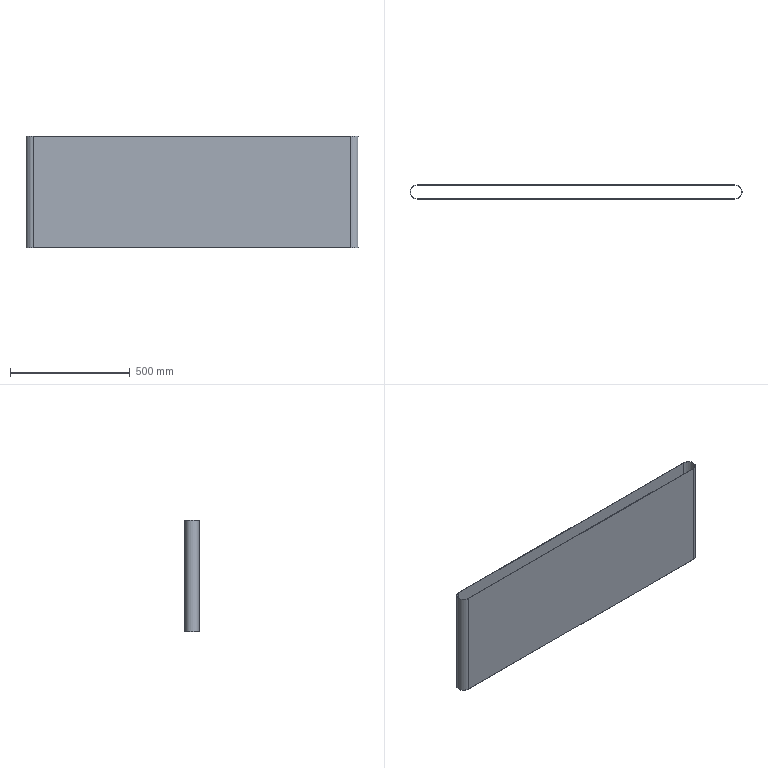Part | STEP file | RUBE 601 | 1 solid | 10 faces | box 1389 x 59.2 x 465 mm | volume 2113671 mm3 | plane 6 | cylinder 4 | commonest cylinder face diameters 56 x2 59.2 x2
STEP:
#1=CARTESIAN_POINT('',(0.,0.,0.));
#2=DIRECTION('',(0.,0.,1.));
#3=DIRECTION('',(1.,0.,0.));
#4=AXIS2_PLACEMENT_3D('',#1,#2,#3);
#5=CARTESIAN_POINT('',(-1248.5,29.6,232.5));
#6=VERTEX_POINT('',#5);
#7=CARTESIAN_POINT('',(-1248.5,-29.6,232.5));
#8=VERTEX_POINT('',#7);
#9=CARTESIAN_POINT('',(-1248.5,0.,232.5));
#10=DIRECTION('',(0.,0.,1.));
#11=DIRECTION('',(1.,0.,0.));
#12=AXIS2_PLACEMENT_3D('',#9,#10,#11);
#13=CIRCLE('',#12,29.6);
#14=CARTESIAN_POINT('',(-1248.5,0.,232.5));
#15=DIRECTION('',(0.,0.,1.));
#16=DIRECTION('',(1.,0.,0.));
#17=AXIS2_PLACEMENT_3D('',#14,#15,#16);
#18=PLANE('',#17);
#19=CARTESIAN_POINT('',(0.,0.));
#20=DIRECTION('',(1.,0.));
#21=AXIS2_PLACEMENT_2D('',#19,#20);
#22=CIRCLE('',#21,29.6);
#23=(GEOMETRIC_REPRESENTATION_CONTEXT(2)PARAMETRIC_REPRESENTATION_CONTEXT()REPRESENTATION_CONTEXT('',''));
#24=DEFINITIONAL_REPRESENTATION('',(#22),#23);
#25=PCURVE('',#18,#24);
#26=CARTESIAN_POINT('',(-1248.5,0.,232.5));
#27=DIRECTION('',(0.,0.,-1.));
#28=DIRECTION('',(-1.,0.,0.));
#29=AXIS2_PLACEMENT_3D('',#26,#27,#28);
#30=CYLINDRICAL_SURFACE('',#29,29.6);
#31=CARTESIAN_POINT('',(3.142,0.));
#32=DIRECTION('',(-1.,0.));
#33=VECTOR('',#32,1.);
#34=LINE('',#31,#33);
#35=(GEOMETRIC_REPRESENTATION_CONTEXT(2)PARAMETRIC_REPRESENTATION_CONTEXT()REPRESENTATION_CONTEXT('',''));
#36=DEFINITIONAL_REPRESENTATION('',(#34),#35);
#37=PCURVE('',#30,#36);
#38=SURFACE_CURVE('',#13,(#25,#37),.PCURVE_S1.);
#39=EDGE_CURVE('',#6,#8,#38,.T.);
#40=ORIENTED_EDGE('',*,*,#39,.T.);
#41=CARTESIAN_POINT('',(81.5,-29.6,232.5));
#42=VERTEX_POINT('',#41);
#43=CARTESIAN_POINT('',(-1248.5,-29.6,232.5));
#44=DIRECTION('',(1.,0.,0.));
#45=VECTOR('',#44,1.);
#46=LINE('',#43,#45);
#47=CARTESIAN_POINT('',(0.,-29.6));
#48=DIRECTION('',(1.,0.));
#49=VECTOR('',#48,1.);
#50=LINE('',#47,#49);
#51=(GEOMETRIC_REPRESENTATION_CONTEXT(2)PARAMETRIC_REPRESENTATION_CONTEXT()REPRESENTATION_CONTEXT('',''));
#52=DEFINITIONAL_REPRESENTATION('',(#50),#51);
#53=PCURVE('',#18,#52);
#54=CARTESIAN_POINT('',(-1248.5,-29.6,232.5));
#55=DIRECTION('',(0.,1.,0.));
#56=DIRECTION('',(-1.,0.,0.));
#57=AXIS2_PLACEMENT_3D('',#54,#55,#56);
#58=PLANE('',#57);
#59=CARTESIAN_POINT('',(0.,0.));
#60=DIRECTION('',(-1.,0.));
#61=VECTOR('',#60,1.);
#62=LINE('',#59,#61);
#63=(GEOMETRIC_REPRESENTATION_CONTEXT(2)PARAMETRIC_REPRESENTATION_CONTEXT()REPRESENTATION_CONTEXT('',''));
#64=DEFINITIONAL_REPRESENTATION('',(#62),#63);
#65=PCURVE('',#58,#64);
#66=SURFACE_CURVE('',#46,(#53,#65),.PCURVE_S1.);
#67=EDGE_CURVE('',#8,#42,#66,.T.);
#68=ORIENTED_EDGE('',*,*,#67,.T.);
#69=CARTESIAN_POINT('',(81.5,29.6,232.5));
#70=VERTEX_POINT('',#69);
#71=CARTESIAN_POINT('',(81.5,0.,232.5));
#72=DIRECTION('',(0.,0.,1.));
#73=DIRECTION('',(1.,0.,0.));
#74=AXIS2_PLACEMENT_3D('',#71,#72,#73);
#75=CIRCLE('',#74,29.6);
#76=CARTESIAN_POINT('',(1330.,0.));
#77=DIRECTION('',(1.,0.));
#78=AXIS2_PLACEMENT_2D('',#76,#77);
#79=CIRCLE('',#78,29.6);
#80=(GEOMETRIC_REPRESENTATION_CONTEXT(2)PARAMETRIC_REPRESENTATION_CONTEXT()REPRESENTATION_CONTEXT('',''));
#81=DEFINITIONAL_REPRESENTATION('',(#79),#80);
#82=PCURVE('',#18,#81);
#83=CARTESIAN_POINT('',(81.5,0.,232.5));
#84=DIRECTION('',(0.,0.,-1.));
#85=DIRECTION('',(-1.,0.,0.));
#86=AXIS2_PLACEMENT_3D('',#83,#84,#85);
#87=CYLINDRICAL_SURFACE('',#86,29.6);
#88=CARTESIAN_POINT('',(9.425,0.));
#89=DIRECTION('',(-1.,0.));
#90=VECTOR('',#89,1.);
#91=LINE('',#88,#90);
#92=(GEOMETRIC_REPRESENTATION_CONTEXT(2)PARAMETRIC_REPRESENTATION_CONTEXT()REPRESENTATION_CONTEXT('',''));
#93=DEFINITIONAL_REPRESENTATION('',(#91),#92);
#94=PCURVE('',#87,#93);
#95=SURFACE_CURVE('',#75,(#82,#94),.PCURVE_S1.);
#96=EDGE_CURVE('',#42,#70,#95,.T.);
#97=ORIENTED_EDGE('',*,*,#96,.T.);
#98=CARTESIAN_POINT('',(-1248.5,29.6,232.5));
#99=DIRECTION('',(-1.,0.,0.));
#100=VECTOR('',#99,1.);
#101=LINE('',#98,#100);
#102=CARTESIAN_POINT('',(0.,29.6));
#103=DIRECTION('',(-1.,0.));
#104=VECTOR('',#103,1.);
#105=LINE('',#102,#104);
#106=(GEOMETRIC_REPRESENTATION_CONTEXT(2)PARAMETRIC_REPRESENTATION_CONTEXT()REPRESENTATION_CONTEXT('',''));
#107=DEFINITIONAL_REPRESENTATION('',(#105),#106);
#108=PCURVE('',#18,#107);
#109=CARTESIAN_POINT('',(-1248.5,29.6,232.5));
#110=DIRECTION('',(0.,-1.,0.));
#111=DIRECTION('',(1.,0.,0.));
#112=AXIS2_PLACEMENT_3D('',#109,#110,#111);
#113=PLANE('',#112);
#114=CARTESIAN_POINT('',(0.,0.));
#115=DIRECTION('',(-1.,0.));
#116=VECTOR('',#115,1.);
#117=LINE('',#114,#116);
#118=(GEOMETRIC_REPRESENTATION_CONTEXT(2)PARAMETRIC_REPRESENTATION_CONTEXT()REPRESENTATION_CONTEXT('',''));
#119=DEFINITIONAL_REPRESENTATION('',(#117),#118);
#120=PCURVE('',#113,#119);
#121=SURFACE_CURVE('',#101,(#108,#120),.PCURVE_S1.);
#122=EDGE_CURVE('',#70,#6,#121,.T.);
#123=ORIENTED_EDGE('',*,*,#122,.T.);
#124=EDGE_LOOP('',(#40,#68,#97,#123));
#125=FACE_BOUND('',#124,.T.);
#126=CARTESIAN_POINT('',(-1248.5,-28.,232.5));
#127=VERTEX_POINT('',#126);
#128=CARTESIAN_POINT('',(81.5,-28.,232.5));
#129=VERTEX_POINT('',#128);
#130=CARTESIAN_POINT('',(-1248.5,-28.,232.5));
#131=DIRECTION('',(1.,0.,0.));
#132=VECTOR('',#131,1.);
#133=LINE('',#130,#132);
#134=CARTESIAN_POINT('',(0.,-28.));
#135=DIRECTION('',(1.,0.));
#136=VECTOR('',#135,1.);
#137=LINE('',#134,#136);
#138=(GEOMETRIC_REPRESENTATION_CONTEXT(2)PARAMETRIC_REPRESENTATION_CONTEXT()REPRESENTATION_CONTEXT('',''));
#139=DEFINITIONAL_REPRESENTATION('',(#137),#138);
#140=PCURVE('',#18,#139);
#141=CARTESIAN_POINT('',(-1248.5,-28.,232.5));
#142=DIRECTION('',(0.,1.,0.));
#143=DIRECTION('',(-1.,0.,0.));
#144=AXIS2_PLACEMENT_3D('',#141,#142,#143);
#145=PLANE('',#144);
#146=CARTESIAN_POINT('',(0.,0.));
#147=DIRECTION('',(-1.,0.));
#148=VECTOR('',#147,1.);
#149=LINE('',#146,#148);
#150=(GEOMETRIC_REPRESENTATION_CONTEXT(2)PARAMETRIC_REPRESENTATION_CONTEXT()REPRESENTATION_CONTEXT('',''));
#151=DEFINITIONAL_REPRESENTATION('',(#149),#150);
#152=PCURVE('',#145,#151);
#153=SURFACE_CURVE('',#133,(#140,#152),.PCURVE_S1.);
#154=EDGE_CURVE('',#127,#129,#153,.T.);
#155=ORIENTED_EDGE('',*,*,#154,.F.);
#156=CARTESIAN_POINT('',(-1248.5,28.,232.5));
#157=VERTEX_POINT('',#156);
#158=CARTESIAN_POINT('',(-1248.5,0.,232.5));
#159=DIRECTION('',(0.,0.,1.));
#160=DIRECTION('',(1.,0.,0.));
#161=AXIS2_PLACEMENT_3D('',#158,#159,#160);
#162=CIRCLE('',#161,28.);
#163=CARTESIAN_POINT('',(0.,0.));
#164=DIRECTION('',(1.,0.));
#165=AXIS2_PLACEMENT_2D('',#163,#164);
#166=CIRCLE('',#165,28.);
#167=(GEOMETRIC_REPRESENTATION_CONTEXT(2)PARAMETRIC_REPRESENTATION_CONTEXT()REPRESENTATION_CONTEXT('',''));
#168=DEFINITIONAL_REPRESENTATION('',(#166),#167);
#169=PCURVE('',#18,#168);
#170=CARTESIAN_POINT('',(-1248.5,0.,232.5));
#171=DIRECTION('',(0.,0.,-1.));
#172=DIRECTION('',(-1.,0.,0.));
#173=AXIS2_PLACEMENT_3D('',#170,#171,#172);
#174=CYLINDRICAL_SURFACE('',#173,28.);
#175=CARTESIAN_POINT('',(9.425,0.));
#176=DIRECTION('',(-1.,0.));
#177=VECTOR('',#176,1.);
#178=LINE('',#175,#177);
#179=(GEOMETRIC_REPRESENTATION_CONTEXT(2)PARAMETRIC_REPRESENTATION_CONTEXT()REPRESENTATION_CONTEXT('',''));
#180=DEFINITIONAL_REPRESENTATION('',(#178),#179);
#181=PCURVE('',#174,#180);
#182=SURFACE_CURVE('',#162,(#169,#181),.PCURVE_S1.);
#183=EDGE_CURVE('',#157,#127,#182,.T.);
#184=ORIENTED_EDGE('',*,*,#183,.F.);
#185=CARTESIAN_POINT('',(81.5,28.,232.5));
#186=VERTEX_POINT('',#185);
#187=CARTESIAN_POINT('',(-1248.5,28.,232.5));
#188=DIRECTION('',(-1.,0.,0.));
#189=VECTOR('',#188,1.);
#190=LINE('',#187,#189);
#191=CARTESIAN_POINT('',(0.,28.));
#192=DIRECTION('',(-1.,0.));
#193=VECTOR('',#192,1.);
#194=LINE('',#191,#193);
#195=(GEOMETRIC_REPRESENTATION_CONTEXT(2)PARAMETRIC_REPRESENTATION_CONTEXT()REPRESENTATION_CONTEXT('',''));
#196=DEFINITIONAL_REPRESENTATION('',(#194),#195);
#197=PCURVE('',#18,#196);
#198=CARTESIAN_POINT('',(-1248.5,28.,232.5));
#199=DIRECTION('',(0.,-1.,0.));
#200=DIRECTION('',(1.,0.,0.));
#201=AXIS2_PLACEMENT_3D('',#198,#199,#200);
#202=PLANE('',#201);
#203=CARTESIAN_POINT('',(0.,0.));
#204=DIRECTION('',(-1.,0.));
#205=VECTOR('',#204,1.);
#206=LINE('',#203,#205);
#207=(GEOMETRIC_REPRESENTATION_CONTEXT(2)PARAMETRIC_REPRESENTATION_CONTEXT()REPRESENTATION_CONTEXT('',''));
#208=DEFINITIONAL_REPRESENTATION('',(#206),#207);
#209=PCURVE('',#202,#208);
#210=SURFACE_CURVE('',#190,(#197,#209),.PCURVE_S1.);
#211=EDGE_CURVE('',#186,#157,#210,.T.);
#212=ORIENTED_EDGE('',*,*,#211,.F.);
#213=CARTESIAN_POINT('',(81.5,0.,232.5));
#214=DIRECTION('',(0.,0.,1.));
#215=DIRECTION('',(1.,0.,0.));
#216=AXIS2_PLACEMENT_3D('',#213,#214,#215);
#217=CIRCLE('',#216,28.);
#218=CARTESIAN_POINT('',(1330.,0.));
#219=DIRECTION('',(1.,0.));
#220=AXIS2_PLACEMENT_2D('',#218,#219);
#221=CIRCLE('',#220,28.);
#222=(GEOMETRIC_REPRESENTATION_CONTEXT(2)PARAMETRIC_REPRESENTATION_CONTEXT()REPRESENTATION_CONTEXT('',''));
#223=DEFINITIONAL_REPRESENTATION('',(#221),#222);
#224=PCURVE('',#18,#223);
#225=CARTESIAN_POINT('',(81.5,0.,232.5));
#226=DIRECTION('',(0.,0.,-1.));
#227=DIRECTION('',(-1.,0.,0.));
#228=AXIS2_PLACEMENT_3D('',#225,#226,#227);
#229=CYLINDRICAL_SURFACE('',#228,28.);
#230=CARTESIAN_POINT('',(9.425,0.));
#231=DIRECTION('',(-1.,0.));
#232=VECTOR('',#231,1.);
#233=LINE('',#230,#232);
#234=(GEOMETRIC_REPRESENTATION_CONTEXT(2)PARAMETRIC_REPRESENTATION_CONTEXT()REPRESENTATION_CONTEXT('',''));
#235=DEFINITIONAL_REPRESENTATION('',(#233),#234);
#236=PCURVE('',#229,#235);
#237=SURFACE_CURVE('',#217,(#224,#236),.PCURVE_S1.);
#238=EDGE_CURVE('',#129,#186,#237,.T.);
#239=ORIENTED_EDGE('',*,*,#238,.F.);
#240=EDGE_LOOP('',(#155,#184,#212,#239));
#241=FACE_BOUND('',#240,.T.);
#242=ADVANCED_FACE('',(#125,#241),#18,.T.);
#243=CARTESIAN_POINT('',(-1248.5,29.6,-232.5));
#244=VERTEX_POINT('',#243);
#245=CARTESIAN_POINT('',(-1248.5,-29.6,-232.5));
#246=VERTEX_POINT('',#245);
#247=CARTESIAN_POINT('',(-1248.5,0.,-232.5));
#248=DIRECTION('',(0.,0.,1.));
#249=DIRECTION('',(1.,0.,0.));
#250=AXIS2_PLACEMENT_3D('',#247,#248,#249);
#251=CIRCLE('',#250,29.6);
#252=CARTESIAN_POINT('',(-1248.5,0.,-232.5));
#253=DIRECTION('',(0.,0.,1.));
#254=DIRECTION('',(1.,0.,0.));
#255=AXIS2_PLACEMENT_3D('',#252,#253,#254);
#256=PLANE('',#255);
#257=CARTESIAN_POINT('',(0.,0.));
#258=DIRECTION('',(1.,0.));
#259=AXIS2_PLACEMENT_2D('',#257,#258);
#260=CIRCLE('',#259,29.6);
#261=(GEOMETRIC_REPRESENTATION_CONTEXT(2)PARAMETRIC_REPRESENTATION_CONTEXT()REPRESENTATION_CONTEXT('',''));
#262=DEFINITIONAL_REPRESENTATION('',(#260),#261);
#263=PCURVE('',#256,#262);
#264=CARTESIAN_POINT('',(3.142,465.));
#265=DIRECTION('',(-1.,0.));
#266=VECTOR('',#265,1.);
#267=LINE('',#264,#266);
#268=(GEOMETRIC_REPRESENTATION_CONTEXT(2)PARAMETRIC_REPRESENTATION_CONTEXT()REPRESENTATION_CONTEXT('',''));
#269=DEFINITIONAL_REPRESENTATION('',(#267),#268);
#270=PCURVE('',#30,#269);
#271=SURFACE_CURVE('',#251,(#263,#270),.PCURVE_S1.);
#272=EDGE_CURVE('',#244,#246,#271,.T.);
#273=ORIENTED_EDGE('',*,*,#272,.F.);
#274=CARTESIAN_POINT('',(81.5,29.6,-232.5));
#275=VERTEX_POINT('',#274);
#276=CARTESIAN_POINT('',(-1248.5,29.6,-232.5));
#277=DIRECTION('',(-1.,0.,0.));
#278=VECTOR('',#277,1.);
#279=LINE('',#276,#278);
#280=CARTESIAN_POINT('',(0.,29.6));
#281=DIRECTION('',(-1.,0.));
#282=VECTOR('',#281,1.);
#283=LINE('',#280,#282);
#284=(GEOMETRIC_REPRESENTATION_CONTEXT(2)PARAMETRIC_REPRESENTATION_CONTEXT()REPRESENTATION_CONTEXT('',''));
#285=DEFINITIONAL_REPRESENTATION('',(#283),#284);
#286=PCURVE('',#256,#285);
#287=CARTESIAN_POINT('',(0.,-465.));
#288=DIRECTION('',(-1.,0.));
#289=VECTOR('',#288,1.);
#290=LINE('',#287,#289);
#291=(GEOMETRIC_REPRESENTATION_CONTEXT(2)PARAMETRIC_REPRESENTATION_CONTEXT()REPRESENTATION_CONTEXT('',''));
#292=DEFINITIONAL_REPRESENTATION('',(#290),#291);
#293=PCURVE('',#113,#292);
#294=SURFACE_CURVE('',#279,(#286,#293),.PCURVE_S1.);
#295=EDGE_CURVE('',#275,#244,#294,.T.);
#296=ORIENTED_EDGE('',*,*,#295,.F.);
#297=CARTESIAN_POINT('',(81.5,-29.6,-232.5));
#298=VERTEX_POINT('',#297);
#299=CARTESIAN_POINT('',(81.5,0.,-232.5));
#300=DIRECTION('',(0.,0.,1.));
#301=DIRECTION('',(1.,0.,0.));
#302=AXIS2_PLACEMENT_3D('',#299,#300,#301);
#303=CIRCLE('',#302,29.6);
#304=CARTESIAN_POINT('',(1330.,0.));
#305=DIRECTION('',(1.,0.));
#306=AXIS2_PLACEMENT_2D('',#304,#305);
#307=CIRCLE('',#306,29.6);
#308=(GEOMETRIC_REPRESENTATION_CONTEXT(2)PARAMETRIC_REPRESENTATION_CONTEXT()REPRESENTATION_CONTEXT('',''));
#309=DEFINITIONAL_REPRESENTATION('',(#307),#308);
#310=PCURVE('',#256,#309);
#311=CARTESIAN_POINT('',(9.425,465.));
#312=DIRECTION('',(-1.,0.));
#313=VECTOR('',#312,1.);
#314=LINE('',#311,#313);
#315=(GEOMETRIC_REPRESENTATION_CONTEXT(2)PARAMETRIC_REPRESENTATION_CONTEXT()REPRESENTATION_CONTEXT('',''));
#316=DEFINITIONAL_REPRESENTATION('',(#314),#315);
#317=PCURVE('',#87,#316);
#318=SURFACE_CURVE('',#303,(#310,#317),.PCURVE_S1.);
#319=EDGE_CURVE('',#298,#275,#318,.T.);
#320=ORIENTED_EDGE('',*,*,#319,.F.);
#321=CARTESIAN_POINT('',(-1248.5,-29.6,-232.5));
#322=DIRECTION('',(1.,0.,0.));
#323=VECTOR('',#322,1.);
#324=LINE('',#321,#323);
#325=CARTESIAN_POINT('',(0.,-29.6));
#326=DIRECTION('',(1.,0.));
#327=VECTOR('',#326,1.);
#328=LINE('',#325,#327);
#329=(GEOMETRIC_REPRESENTATION_CONTEXT(2)PARAMETRIC_REPRESENTATION_CONTEXT()REPRESENTATION_CONTEXT('',''));
#330=DEFINITIONAL_REPRESENTATION('',(#328),#329);
#331=PCURVE('',#256,#330);
#332=CARTESIAN_POINT('',(0.,-465.));
#333=DIRECTION('',(-1.,0.));
#334=VECTOR('',#333,1.);
#335=LINE('',#332,#334);
#336=(GEOMETRIC_REPRESENTATION_CONTEXT(2)PARAMETRIC_REPRESENTATION_CONTEXT()REPRESENTATION_CONTEXT('',''));
#337=DEFINITIONAL_REPRESENTATION('',(#335),#336);
#338=PCURVE('',#58,#337);
#339=SURFACE_CURVE('',#324,(#331,#338),.PCURVE_S1.);
#340=EDGE_CURVE('',#246,#298,#339,.T.);
#341=ORIENTED_EDGE('',*,*,#340,.F.);
#342=EDGE_LOOP('',(#273,#296,#320,#341));
#343=FACE_BOUND('',#342,.T.);
#344=CARTESIAN_POINT('',(-1248.5,28.,-232.5));
#345=VERTEX_POINT('',#344);
#346=CARTESIAN_POINT('',(-1248.5,-28.,-232.5));
#347=VERTEX_POINT('',#346);
#348=CARTESIAN_POINT('',(-1248.5,0.,-232.5));
#349=DIRECTION('',(0.,0.,1.));
#350=DIRECTION('',(1.,0.,0.));
#351=AXIS2_PLACEMENT_3D('',#348,#349,#350);
#352=CIRCLE('',#351,28.);
#353=CARTESIAN_POINT('',(0.,0.));
#354=DIRECTION('',(1.,0.));
#355=AXIS2_PLACEMENT_2D('',#353,#354);
#356=CIRCLE('',#355,28.);
#357=(GEOMETRIC_REPRESENTATION_CONTEXT(2)PARAMETRIC_REPRESENTATION_CONTEXT()REPRESENTATION_CONTEXT('',''));
#358=DEFINITIONAL_REPRESENTATION('',(#356),#357);
#359=PCURVE('',#256,#358);
#360=CARTESIAN_POINT('',(9.425,465.));
#361=DIRECTION('',(-1.,0.));
#362=VECTOR('',#361,1.);
#363=LINE('',#360,#362);
#364=(GEOMETRIC_REPRESENTATION_CONTEXT(2)PARAMETRIC_REPRESENTATION_CONTEXT()REPRESENTATION_CONTEXT('',''));
#365=DEFINITIONAL_REPRESENTATION('',(#363),#364);
#366=PCURVE('',#174,#365);
#367=SURFACE_CURVE('',#352,(#359,#366),.PCURVE_S1.);
#368=EDGE_CURVE('',#345,#347,#367,.T.);
#369=ORIENTED_EDGE('',*,*,#368,.T.);
#370=CARTESIAN_POINT('',(81.5,-28.,-232.5));
#371=VERTEX_POINT('',#370);
#372=CARTESIAN_POINT('',(-1248.5,-28.,-232.5));
#373=DIRECTION('',(1.,0.,0.));
#374=VECTOR('',#373,1.);
#375=LINE('',#372,#374);
#376=CARTESIAN_POINT('',(0.,-28.));
#377=DIRECTION('',(1.,0.));
#378=VECTOR('',#377,1.);
#379=LINE('',#376,#378);
#380=(GEOMETRIC_REPRESENTATION_CONTEXT(2)PARAMETRIC_REPRESENTATION_CONTEXT()REPRESENTATION_CONTEXT('',''));
#381=DEFINITIONAL_REPRESENTATION('',(#379),#380);
#382=PCURVE('',#256,#381);
#383=CARTESIAN_POINT('',(0.,-465.));
#384=DIRECTION('',(-1.,0.));
#385=VECTOR('',#384,1.);
#386=LINE('',#383,#385);
#387=(GEOMETRIC_REPRESENTATION_CONTEXT(2)PARAMETRIC_REPRESENTATION_CONTEXT()REPRESENTATION_CONTEXT('',''));
#388=DEFINITIONAL_REPRESENTATION('',(#386),#387);
#389=PCURVE('',#145,#388);
#390=SURFACE_CURVE('',#375,(#382,#389),.PCURVE_S1.);
#391=EDGE_CURVE('',#347,#371,#390,.T.);
#392=ORIENTED_EDGE('',*,*,#391,.T.);
#393=CARTESIAN_POINT('',(81.5,28.,-232.5));
#394=VERTEX_POINT('',#393);
#395=CARTESIAN_POINT('',(81.5,0.,-232.5));
#396=DIRECTION('',(0.,0.,1.));
#397=DIRECTION('',(1.,0.,0.));
#398=AXIS2_PLACEMENT_3D('',#395,#396,#397);
#399=CIRCLE('',#398,28.);
#400=CARTESIAN_POINT('',(1330.,0.));
#401=DIRECTION('',(1.,0.));
#402=AXIS2_PLACEMENT_2D('',#400,#401);
#403=CIRCLE('',#402,28.);
#404=(GEOMETRIC_REPRESENTATION_CONTEXT(2)PARAMETRIC_REPRESENTATION_CONTEXT()REPRESENTATION_CONTEXT('',''));
#405=DEFINITIONAL_REPRESENTATION('',(#403),#404);
#406=PCURVE('',#256,#405);
#407=CARTESIAN_POINT('',(9.425,465.));
#408=DIRECTION('',(-1.,0.));
#409=VECTOR('',#408,1.);
#410=LINE('',#407,#409);
#411=(GEOMETRIC_REPRESENTATION_CONTEXT(2)PARAMETRIC_REPRESENTATION_CONTEXT()REPRESENTATION_CONTEXT('',''));
#412=DEFINITIONAL_REPRESENTATION('',(#410),#411);
#413=PCURVE('',#229,#412);
#414=SURFACE_CURVE('',#399,(#406,#413),.PCURVE_S1.);
#415=EDGE_CURVE('',#371,#394,#414,.T.);
#416=ORIENTED_EDGE('',*,*,#415,.T.);
#417=CARTESIAN_POINT('',(-1248.5,28.,-232.5));
#418=DIRECTION('',(-1.,0.,0.));
#419=VECTOR('',#418,1.);
#420=LINE('',#417,#419);
#421=CARTESIAN_POINT('',(0.,28.));
#422=DIRECTION('',(-1.,0.));
#423=VECTOR('',#422,1.);
#424=LINE('',#421,#423);
#425=(GEOMETRIC_REPRESENTATION_CONTEXT(2)PARAMETRIC_REPRESENTATION_CONTEXT()REPRESENTATION_CONTEXT('',''));
#426=DEFINITIONAL_REPRESENTATION('',(#424),#425);
#427=PCURVE('',#256,#426);
#428=CARTESIAN_POINT('',(0.,-465.));
#429=DIRECTION('',(-1.,0.));
#430=VECTOR('',#429,1.);
#431=LINE('',#428,#430);
#432=(GEOMETRIC_REPRESENTATION_CONTEXT(2)PARAMETRIC_REPRESENTATION_CONTEXT()REPRESENTATION_CONTEXT('',''));
#433=DEFINITIONAL_REPRESENTATION('',(#431),#432);
#434=PCURVE('',#202,#433);
#435=SURFACE_CURVE('',#420,(#427,#434),.PCURVE_S1.);
#436=EDGE_CURVE('',#394,#345,#435,.T.);
#437=ORIENTED_EDGE('',*,*,#436,.T.);
#438=EDGE_LOOP('',(#369,#392,#416,#437));
#439=FACE_BOUND('',#438,.T.);
#440=ADVANCED_FACE('',(#343,#439),#256,.F.);
#441=ORIENTED_EDGE('',*,*,#272,.T.);
#442=CARTESIAN_POINT('',(-1248.5,-29.6,232.5));
#443=DIRECTION('',(0.,0.,-1.));
#444=VECTOR('',#443,1.);
#445=LINE('',#442,#444);
#446=CARTESIAN_POINT('',(-1.571,0.));
#447=DIRECTION('',(0.,1.));
#448=VECTOR('',#447,1.);
#449=LINE('',#446,#448);
#450=(GEOMETRIC_REPRESENTATION_CONTEXT(2)PARAMETRIC_REPRESENTATION_CONTEXT()REPRESENTATION_CONTEXT('',''));
#451=DEFINITIONAL_REPRESENTATION('',(#449),#450);
#452=PCURVE('',#30,#451);
#453=CARTESIAN_POINT('',(0.,0.));
#454=DIRECTION('',(0.,-1.));
#455=VECTOR('',#454,1.);
#456=LINE('',#453,#455);
#457=(GEOMETRIC_REPRESENTATION_CONTEXT(2)PARAMETRIC_REPRESENTATION_CONTEXT()REPRESENTATION_CONTEXT('',''));
#458=DEFINITIONAL_REPRESENTATION('',(#456),#457);
#459=PCURVE('',#58,#458);
#460=SURFACE_CURVE('',#445,(#452,#459),.PCURVE_S1.);
#461=EDGE_CURVE('',#8,#246,#460,.T.);
#462=ORIENTED_EDGE('',*,*,#461,.F.);
#463=ORIENTED_EDGE('',*,*,#39,.F.);
#464=CARTESIAN_POINT('',(-1248.5,29.6,232.5));
#465=DIRECTION('',(0.,0.,-1.));
#466=VECTOR('',#465,1.);
#467=LINE('',#464,#466);
#468=CARTESIAN_POINT('',(1.571,0.));
#469=DIRECTION('',(0.,1.));
#470=VECTOR('',#469,1.);
#471=LINE('',#468,#470);
#472=(GEOMETRIC_REPRESENTATION_CONTEXT(2)PARAMETRIC_REPRESENTATION_CONTEXT()REPRESENTATION_CONTEXT('',''));
#473=DEFINITIONAL_REPRESENTATION('',(#471),#472);
#474=PCURVE('',#30,#473);
#475=CARTESIAN_POINT('',(0.,0.));
#476=DIRECTION('',(0.,-1.));
#477=VECTOR('',#476,1.);
#478=LINE('',#475,#477);
#479=(GEOMETRIC_REPRESENTATION_CONTEXT(2)PARAMETRIC_REPRESENTATION_CONTEXT()REPRESENTATION_CONTEXT('',''));
#480=DEFINITIONAL_REPRESENTATION('',(#478),#479);
#481=PCURVE('',#113,#480);
#482=SURFACE_CURVE('',#467,(#474,#481),.PCURVE_S1.);
#483=EDGE_CURVE('',#6,#244,#482,.T.);
#484=ORIENTED_EDGE('',*,*,#483,.T.);
#485=EDGE_LOOP('',(#441,#462,#463,#484));
#486=FACE_BOUND('',#485,.T.);
#487=ADVANCED_FACE('',(#486),#30,.T.);
#488=ORIENTED_EDGE('',*,*,#340,.T.);
#489=CARTESIAN_POINT('',(81.5,-29.6,232.5));
#490=DIRECTION('',(0.,0.,-1.));
#491=VECTOR('',#490,1.);
#492=LINE('',#489,#491);
#493=CARTESIAN_POINT('',(-1330.,0.));
#494=DIRECTION('',(0.,-1.));
#495=VECTOR('',#494,1.);
#496=LINE('',#493,#495);
#497=(GEOMETRIC_REPRESENTATION_CONTEXT(2)PARAMETRIC_REPRESENTATION_CONTEXT()REPRESENTATION_CONTEXT('',''));
#498=DEFINITIONAL_REPRESENTATION('',(#496),#497);
#499=PCURVE('',#58,#498);
#500=CARTESIAN_POINT('',(4.712,0.));
#501=DIRECTION('',(0.,1.));
#502=VECTOR('',#501,1.);
#503=LINE('',#500,#502);
#504=(GEOMETRIC_REPRESENTATION_CONTEXT(2)PARAMETRIC_REPRESENTATION_CONTEXT()REPRESENTATION_CONTEXT('',''));
#505=DEFINITIONAL_REPRESENTATION('',(#503),#504);
#506=PCURVE('',#87,#505);
#507=SURFACE_CURVE('',#492,(#499,#506),.PCURVE_S1.);
#508=EDGE_CURVE('',#42,#298,#507,.T.);
#509=ORIENTED_EDGE('',*,*,#508,.F.);
#510=ORIENTED_EDGE('',*,*,#67,.F.);
#511=ORIENTED_EDGE('',*,*,#461,.T.);
#512=EDGE_LOOP('',(#488,#509,#510,#511));
#513=FACE_BOUND('',#512,.T.);
#514=ADVANCED_FACE('',(#513),#58,.F.);
#515=ORIENTED_EDGE('',*,*,#319,.T.);
#516=CARTESIAN_POINT('',(81.5,29.6,232.5));
#517=DIRECTION('',(0.,0.,-1.));
#518=VECTOR('',#517,1.);
#519=LINE('',#516,#518);
#520=CARTESIAN_POINT('',(1.571,0.));
#521=DIRECTION('',(0.,1.));
#522=VECTOR('',#521,1.);
#523=LINE('',#520,#522);
#524=(GEOMETRIC_REPRESENTATION_CONTEXT(2)PARAMETRIC_REPRESENTATION_CONTEXT()REPRESENTATION_CONTEXT('',''));
#525=DEFINITIONAL_REPRESENTATION('',(#523),#524);
#526=PCURVE('',#87,#525);
#527=CARTESIAN_POINT('',(1330.,0.));
#528=DIRECTION('',(0.,-1.));
#529=VECTOR('',#528,1.);
#530=LINE('',#527,#529);
#531=(GEOMETRIC_REPRESENTATION_CONTEXT(2)PARAMETRIC_REPRESENTATION_CONTEXT()REPRESENTATION_CONTEXT('',''));
#532=DEFINITIONAL_REPRESENTATION('',(#530),#531);
#533=PCURVE('',#113,#532);
#534=SURFACE_CURVE('',#519,(#526,#533),.PCURVE_S1.);
#535=EDGE_CURVE('',#70,#275,#534,.T.);
#536=ORIENTED_EDGE('',*,*,#535,.F.);
#537=ORIENTED_EDGE('',*,*,#96,.F.);
#538=ORIENTED_EDGE('',*,*,#508,.T.);
#539=EDGE_LOOP('',(#515,#536,#537,#538));
#540=FACE_BOUND('',#539,.T.);
#541=ADVANCED_FACE('',(#540),#87,.T.);
#542=ORIENTED_EDGE('',*,*,#295,.T.);
#543=ORIENTED_EDGE('',*,*,#483,.F.);
#544=ORIENTED_EDGE('',*,*,#122,.F.);
#545=ORIENTED_EDGE('',*,*,#535,.T.);
#546=EDGE_LOOP('',(#542,#543,#544,#545));
#547=FACE_BOUND('',#546,.T.);
#548=ADVANCED_FACE('',(#547),#113,.F.);
#549=CARTESIAN_POINT('',(-1248.5,-28.,232.5));
#550=DIRECTION('',(0.,0.,-1.));
#551=VECTOR('',#550,1.);
#552=LINE('',#549,#551);
#553=CARTESIAN_POINT('',(4.712,0.));
#554=DIRECTION('',(0.,1.));
#555=VECTOR('',#554,1.);
#556=LINE('',#553,#555);
#557=(GEOMETRIC_REPRESENTATION_CONTEXT(2)PARAMETRIC_REPRESENTATION_CONTEXT()REPRESENTATION_CONTEXT('',''));
#558=DEFINITIONAL_REPRESENTATION('',(#556),#557);
#559=PCURVE('',#174,#558);
#560=CARTESIAN_POINT('',(0.,0.));
#561=DIRECTION('',(0.,-1.));
#562=VECTOR('',#561,1.);
#563=LINE('',#560,#562);
#564=(GEOMETRIC_REPRESENTATION_CONTEXT(2)PARAMETRIC_REPRESENTATION_CONTEXT()REPRESENTATION_CONTEXT('',''));
#565=DEFINITIONAL_REPRESENTATION('',(#563),#564);
#566=PCURVE('',#145,#565);
#567=SURFACE_CURVE('',#552,(#559,#566),.PCURVE_S1.);
#568=EDGE_CURVE('',#127,#347,#567,.T.);
#569=ORIENTED_EDGE('',*,*,#568,.F.);
#570=ORIENTED_EDGE('',*,*,#183,.F.);
#571=CARTESIAN_POINT('',(-1248.5,28.,232.5));
#572=DIRECTION('',(0.,0.,-1.));
#573=VECTOR('',#572,1.);
#574=LINE('',#571,#573);
#575=CARTESIAN_POINT('',(7.854,0.));
#576=DIRECTION('',(0.,1.));
#577=VECTOR('',#576,1.);
#578=LINE('',#575,#577);
#579=(GEOMETRIC_REPRESENTATION_CONTEXT(2)PARAMETRIC_REPRESENTATION_CONTEXT()REPRESENTATION_CONTEXT('',''));
#580=DEFINITIONAL_REPRESENTATION('',(#578),#579);
#581=PCURVE('',#174,#580);
#582=CARTESIAN_POINT('',(0.,0.));
#583=DIRECTION('',(0.,-1.));
#584=VECTOR('',#583,1.);
#585=LINE('',#582,#584);
#586=(GEOMETRIC_REPRESENTATION_CONTEXT(2)PARAMETRIC_REPRESENTATION_CONTEXT()REPRESENTATION_CONTEXT('',''));
#587=DEFINITIONAL_REPRESENTATION('',(#585),#586);
#588=PCURVE('',#202,#587);
#589=SURFACE_CURVE('',#574,(#581,#588),.PCURVE_S1.);
#590=EDGE_CURVE('',#157,#345,#589,.T.);
#591=ORIENTED_EDGE('',*,*,#590,.T.);
#592=ORIENTED_EDGE('',*,*,#368,.T.);
#593=EDGE_LOOP('',(#569,#570,#591,#592));
#594=FACE_BOUND('',#593,.F.);
#595=ADVANCED_FACE('',(#594),#174,.F.);
#596=ORIENTED_EDGE('',*,*,#391,.F.);
#597=ORIENTED_EDGE('',*,*,#568,.F.);
#598=ORIENTED_EDGE('',*,*,#154,.T.);
#599=CARTESIAN_POINT('',(81.5,-28.,232.5));
#600=DIRECTION('',(0.,0.,-1.));
#601=VECTOR('',#600,1.);
#602=LINE('',#599,#601);
#603=CARTESIAN_POINT('',(-1330.,0.));
#604=DIRECTION('',(0.,-1.));
#605=VECTOR('',#604,1.);
#606=LINE('',#603,#605);
#607=(GEOMETRIC_REPRESENTATION_CONTEXT(2)PARAMETRIC_REPRESENTATION_CONTEXT()REPRESENTATION_CONTEXT('',''));
#608=DEFINITIONAL_REPRESENTATION('',(#606),#607);
#609=PCURVE('',#145,#608);
#610=CARTESIAN_POINT('',(4.712,0.));
#611=DIRECTION('',(0.,1.));
#612=VECTOR('',#611,1.);
#613=LINE('',#610,#612);
#614=(GEOMETRIC_REPRESENTATION_CONTEXT(2)PARAMETRIC_REPRESENTATION_CONTEXT()REPRESENTATION_CONTEXT('',''));
#615=DEFINITIONAL_REPRESENTATION('',(#613),#614);
#616=PCURVE('',#229,#615);
#617=SURFACE_CURVE('',#602,(#609,#616),.PCURVE_S1.);
#618=EDGE_CURVE('',#129,#371,#617,.T.);
#619=ORIENTED_EDGE('',*,*,#618,.T.);
#620=EDGE_LOOP('',(#596,#597,#598,#619));
#621=FACE_BOUND('',#620,.T.);
#622=ADVANCED_FACE('',(#621),#145,.T.);
#623=CARTESIAN_POINT('',(81.5,28.,232.5));
#624=DIRECTION('',(0.,0.,-1.));
#625=VECTOR('',#624,1.);
#626=LINE('',#623,#625);
#627=CARTESIAN_POINT('',(1.571,0.));
#628=DIRECTION('',(0.,1.));
#629=VECTOR('',#628,1.);
#630=LINE('',#627,#629);
#631=(GEOMETRIC_REPRESENTATION_CONTEXT(2)PARAMETRIC_REPRESENTATION_CONTEXT()REPRESENTATION_CONTEXT('',''));
#632=DEFINITIONAL_REPRESENTATION('',(#630),#631);
#633=PCURVE('',#229,#632);
#634=CARTESIAN_POINT('',(1330.,0.));
#635=DIRECTION('',(0.,-1.));
#636=VECTOR('',#635,1.);
#637=LINE('',#634,#636);
#638=(GEOMETRIC_REPRESENTATION_CONTEXT(2)PARAMETRIC_REPRESENTATION_CONTEXT()REPRESENTATION_CONTEXT('',''));
#639=DEFINITIONAL_REPRESENTATION('',(#637),#638);
#640=PCURVE('',#202,#639);
#641=SURFACE_CURVE('',#626,(#633,#640),.PCURVE_S1.);
#642=EDGE_CURVE('',#186,#394,#641,.T.);
#643=ORIENTED_EDGE('',*,*,#642,.F.);
#644=ORIENTED_EDGE('',*,*,#238,.F.);
#645=ORIENTED_EDGE('',*,*,#618,.T.);
#646=ORIENTED_EDGE('',*,*,#415,.T.);
#647=EDGE_LOOP('',(#643,#644,#645,#646));
#648=FACE_BOUND('',#647,.F.);
#649=ADVANCED_FACE('',(#648),#229,.F.);
#650=ORIENTED_EDGE('',*,*,#436,.F.);
#651=ORIENTED_EDGE('',*,*,#642,.F.);
#652=ORIENTED_EDGE('',*,*,#211,.T.);
#653=ORIENTED_EDGE('',*,*,#590,.T.);
#654=EDGE_LOOP('',(#650,#651,#652,#653));
#655=FACE_BOUND('',#654,.T.);
#656=ADVANCED_FACE('',(#655),#202,.T.);
#657=CLOSED_SHELL('',(#242,#440,#487,#514,#541,#548,#595,#622,#649,#656));
#658=MANIFOLD_SOLID_BREP('',#657);
#659=(LENGTH_UNIT()NAMED_UNIT(*)SI_UNIT(.MILLI.,.METRE.));
#660=UNCERTAINTY_MEASURE_WITH_UNIT(LENGTH_MEASURE(0.0000001),#659,'','');
#661=(NAMED_UNIT(*)PLANE_ANGLE_UNIT()SI_UNIT($,.RADIAN.));
#662=(NAMED_UNIT(*)SI_UNIT($,.STERADIAN.)SOLID_ANGLE_UNIT());
#663=(GEOMETRIC_REPRESENTATION_CONTEXT(3)GLOBAL_UNCERTAINTY_ASSIGNED_CONTEXT((#660))GLOBAL_UNIT_ASSIGNED_CONTEXT((#659,#661,#662))REPRESENTATION_CONTEXT('',''));
#664=ADVANCED_BREP_SHAPE_REPRESENTATION('',(#4,#658),#663);